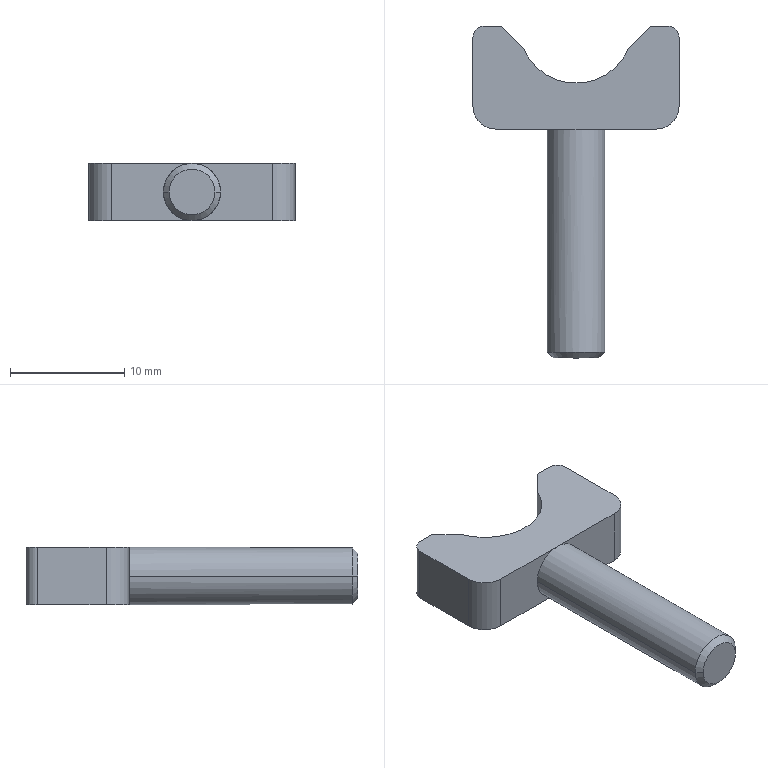Part | SolidWorks | features Chamfer 2, Fillet 2, ICE 2, Extrusion 1 | 1 solid | 20 faces | box 18 x 29 x 5 mm | volume 980.993 mm3 | plane 11 | cylinder 7 | cone 2 | commonest cylinder face diameters 2 x2 4 x2 5 x2 10 x1
STEP:
#1=CARTESIAN_POINT('',(2.,-29.,0.));
#2=VERTEX_POINT('',#1);
#3=CARTESIAN_POINT('',(-2.,-29.,0.));
#4=VERTEX_POINT('',#3);
#5=CARTESIAN_POINT('',(0.,-29.,0.));
#6=DIRECTION('',(0.,-1.,0.));
#7=DIRECTION('',(1.,0.,0.));
#8=AXIS2_PLACEMENT_3D('',#5,#6,#7);
#9=CIRCLE('',#8,2.);
#10=EDGE_CURVE('',#2,#4,#9,.T.);
#11=ORIENTED_EDGE('',*,*,#10,.F.);
#12=CARTESIAN_POINT('',(2.5,-28.5,0.));
#13=VERTEX_POINT('',#12);
#14=CARTESIAN_POINT('',(2.,-29.,0.));
#15=DIRECTION('',(0.7071,0.7071,0.));
#16=VECTOR('',#15,1000.);
#17=LINE('',#14,#16);
#18=EDGE_CURVE('',#2,#13,#17,.T.);
#19=ORIENTED_EDGE('',*,*,#18,.T.);
#20=CARTESIAN_POINT('',(-2.5,-28.5,0.));
#21=VERTEX_POINT('',#20);
#22=CARTESIAN_POINT('',(0.,-28.5,0.));
#23=DIRECTION('',(0.,1.,0.));
#24=DIRECTION('',(1.,0.,0.));
#25=AXIS2_PLACEMENT_3D('',#22,#23,#24);
#26=CIRCLE('',#25,2.5);
#27=EDGE_CURVE('',#21,#13,#26,.T.);
#28=ORIENTED_EDGE('',*,*,#27,.F.);
#29=CARTESIAN_POINT('',(-2.,-29.,0.));
#30=DIRECTION('',(-0.7071,0.7071,0.));
#31=VECTOR('',#30,1000.);
#32=LINE('',#29,#31);
#33=EDGE_CURVE('',#4,#21,#32,.T.);
#34=ORIENTED_EDGE('',*,*,#33,.F.);
#35=EDGE_LOOP('',(#11,#19,#28,#34));
#36=FACE_OUTER_BOUND('',#35,.T.);
#37=CARTESIAN_POINT('',(0.,-29.,0.));
#38=DIRECTION('',(0.,1.,0.));
#39=DIRECTION('',(-1.,0.,0.));
#40=AXIS2_PLACEMENT_3D('',#37,#38,#39);
#41=CONICAL_SURFACE('',#40,2.,0.7854);
#42=ADVANCED_FACE('',(#36),#41,.T.);
#43=ORIENTED_EDGE('',*,*,#27,.T.);
#44=CARTESIAN_POINT('',(2.5,-9.,0.));
#45=VERTEX_POINT('',#44);
#46=CARTESIAN_POINT('',(2.5,-29.,0.));
#47=DIRECTION('',(0.,1.,0.));
#48=VECTOR('',#47,1000.);
#49=LINE('',#46,#48);
#50=EDGE_CURVE('',#13,#45,#49,.T.);
#51=ORIENTED_EDGE('',*,*,#50,.T.);
#52=CARTESIAN_POINT('',(0.,-9.,2.5));
#53=VERTEX_POINT('',#52);
#54=CARTESIAN_POINT('',(0.,-9.,0.));
#55=DIRECTION('',(0.,-1.,0.));
#56=DIRECTION('',(1.,0.,0.));
#57=AXIS2_PLACEMENT_3D('',#54,#55,#56);
#58=CIRCLE('',#57,2.5);
#59=EDGE_CURVE('',#45,#53,#58,.T.);
#60=ORIENTED_EDGE('',*,*,#59,.T.);
#61=CARTESIAN_POINT('',(-2.5,-9.,0.));
#62=VERTEX_POINT('',#61);
#63=CARTESIAN_POINT('',(0.,-9.,0.));
#64=DIRECTION('',(0.,-1.,0.));
#65=DIRECTION('',(1.,0.,0.));
#66=AXIS2_PLACEMENT_3D('',#63,#64,#65);
#67=CIRCLE('',#66,2.5);
#68=EDGE_CURVE('',#53,#62,#67,.T.);
#69=ORIENTED_EDGE('',*,*,#68,.T.);
#70=CARTESIAN_POINT('',(-2.5,-29.,0.));
#71=DIRECTION('',(0.,1.,0.));
#72=VECTOR('',#71,1000.);
#73=LINE('',#70,#72);
#74=EDGE_CURVE('',#21,#62,#73,.T.);
#75=ORIENTED_EDGE('',*,*,#74,.F.);
#76=EDGE_LOOP('',(#43,#51,#60,#69,#75));
#77=FACE_OUTER_BOUND('',#76,.T.);
#78=CARTESIAN_POINT('',(0.,-29.,0.));
#79=DIRECTION('',(0.,1.,0.));
#80=DIRECTION('',(-1.,0.,0.));
#81=AXIS2_PLACEMENT_3D('',#78,#79,#80);
#82=CYLINDRICAL_SURFACE('',#81,2.5);
#83=ADVANCED_FACE('',(#77),#82,.T.);
#84=CARTESIAN_POINT('',(-7.,-9.,2.5));
#85=VERTEX_POINT('',#84);
#86=CARTESIAN_POINT('',(9.,-9.,2.5));
#87=DIRECTION('',(1.,0.,0.));
#88=VECTOR('',#87,1000.);
#89=LINE('',#86,#88);
#90=EDGE_CURVE('',#85,#53,#89,.T.);
#91=ORIENTED_EDGE('',*,*,#90,.F.);
#92=CARTESIAN_POINT('',(-7.,-9.,-2.5));
#93=VERTEX_POINT('',#92);
#94=CARTESIAN_POINT('',(-7.,-9.,2.5));
#95=DIRECTION('',(0.,0.,-1.));
#96=VECTOR('',#95,1000.);
#97=LINE('',#94,#96);
#98=EDGE_CURVE('',#85,#93,#97,.T.);
#99=ORIENTED_EDGE('',*,*,#98,.T.);
#100=CARTESIAN_POINT('',(0.,-9.,-2.5));
#101=VERTEX_POINT('',#100);
#102=CARTESIAN_POINT('',(9.,-9.,-2.5));
#103=DIRECTION('',(1.,0.,0.));
#104=VECTOR('',#103,1000.);
#105=LINE('',#102,#104);
#106=EDGE_CURVE('',#93,#101,#105,.T.);
#107=ORIENTED_EDGE('',*,*,#106,.T.);
#108=CARTESIAN_POINT('',(0.,-9.,0.));
#109=DIRECTION('',(0.,-1.,0.));
#110=DIRECTION('',(1.,0.,0.));
#111=AXIS2_PLACEMENT_3D('',#108,#109,#110);
#112=CIRCLE('',#111,2.5);
#113=EDGE_CURVE('',#62,#101,#112,.T.);
#114=ORIENTED_EDGE('',*,*,#113,.F.);
#115=ORIENTED_EDGE('',*,*,#68,.F.);
#116=EDGE_LOOP('',(#91,#99,#107,#114,#115));
#117=FACE_OUTER_BOUND('',#116,.T.);
#118=CARTESIAN_POINT('',(9.,-9.,2.5));
#119=DIRECTION('',(0.,1.,0.));
#120=DIRECTION('',(-1.,0.,0.));
#121=AXIS2_PLACEMENT_3D('',#118,#119,#120);
#122=PLANE('',#121);
#123=ADVANCED_FACE('',(#117),#122,.F.);
#124=CARTESIAN_POINT('',(9.,-7.,2.5));
#125=VERTEX_POINT('',#124);
#126=CARTESIAN_POINT('',(9.,-1.,2.5));
#127=VERTEX_POINT('',#126);
#128=CARTESIAN_POINT('',(9.,-9.,2.5));
#129=DIRECTION('',(0.,1.,0.));
#130=VECTOR('',#129,1000.);
#131=LINE('',#128,#130);
#132=EDGE_CURVE('',#125,#127,#131,.T.);
#133=ORIENTED_EDGE('',*,*,#132,.T.);
#134=CARTESIAN_POINT('',(8.,0.,2.5));
#135=VERTEX_POINT('',#134);
#136=CARTESIAN_POINT('',(8.,-1.,2.5));
#137=DIRECTION('',(0.,0.,1.));
#138=DIRECTION('',(1.,0.,0.));
#139=AXIS2_PLACEMENT_3D('',#136,#137,#138);
#140=CIRCLE('',#139,1.);
#141=EDGE_CURVE('',#127,#135,#140,.T.);
#142=ORIENTED_EDGE('',*,*,#141,.T.);
#143=CARTESIAN_POINT('',(6.5,0.,2.5));
#144=VERTEX_POINT('',#143);
#145=CARTESIAN_POINT('',(-9.,0.,2.5));
#146=DIRECTION('',(1.,0.,0.));
#147=VECTOR('',#146,1000.);
#148=LINE('',#145,#147);
#149=EDGE_CURVE('',#144,#135,#148,.T.);
#150=ORIENTED_EDGE('',*,*,#149,.F.);
#151=CARTESIAN_POINT('',(4.642,-1.858,2.5));
#152=VERTEX_POINT('',#151);
#153=CARTESIAN_POINT('',(3.25,-3.25,2.5));
#154=DIRECTION('',(-0.7071,-0.7071,0.));
#155=VECTOR('',#154,1000.);
#156=LINE('',#153,#155);
#157=EDGE_CURVE('',#144,#152,#156,.T.);
#158=ORIENTED_EDGE('',*,*,#157,.T.);
#159=CARTESIAN_POINT('',(-4.642,-1.858,2.5));
#160=VERTEX_POINT('',#159);
#161=CARTESIAN_POINT('',(0.,0.,2.5));
#162=DIRECTION('',(0.,0.,1.));
#163=DIRECTION('',(1.,0.,0.));
#164=AXIS2_PLACEMENT_3D('',#161,#162,#163);
#165=CIRCLE('',#164,5.);
#166=EDGE_CURVE('',#160,#152,#165,.T.);
#167=ORIENTED_EDGE('',*,*,#166,.F.);
#168=CARTESIAN_POINT('',(-6.5,0.,2.5));
#169=VERTEX_POINT('',#168);
#170=CARTESIAN_POINT('',(-3.25,-3.25,2.5));
#171=DIRECTION('',(-0.7071,0.7071,0.));
#172=VECTOR('',#171,1000.);
#173=LINE('',#170,#172);
#174=EDGE_CURVE('',#160,#169,#173,.T.);
#175=ORIENTED_EDGE('',*,*,#174,.T.);
#176=CARTESIAN_POINT('',(-8.,0.,2.5));
#177=VERTEX_POINT('',#176);
#178=CARTESIAN_POINT('',(-9.,0.,2.5));
#179=DIRECTION('',(1.,0.,0.));
#180=VECTOR('',#179,1000.);
#181=LINE('',#178,#180);
#182=EDGE_CURVE('',#177,#169,#181,.T.);
#183=ORIENTED_EDGE('',*,*,#182,.F.);
#184=CARTESIAN_POINT('',(-9.,-1.,2.5));
#185=VERTEX_POINT('',#184);
#186=CARTESIAN_POINT('',(-8.,-1.,2.5));
#187=DIRECTION('',(0.,0.,1.));
#188=DIRECTION('',(1.,0.,0.));
#189=AXIS2_PLACEMENT_3D('',#186,#187,#188);
#190=CIRCLE('',#189,1.);
#191=EDGE_CURVE('',#177,#185,#190,.T.);
#192=ORIENTED_EDGE('',*,*,#191,.T.);
#193=CARTESIAN_POINT('',(-9.,-7.,2.5));
#194=VERTEX_POINT('',#193);
#195=CARTESIAN_POINT('',(-9.,-9.,2.5));
#196=DIRECTION('',(0.,-1.,0.));
#197=VECTOR('',#196,1000.);
#198=LINE('',#195,#197);
#199=EDGE_CURVE('',#185,#194,#198,.T.);
#200=ORIENTED_EDGE('',*,*,#199,.T.);
#201=CARTESIAN_POINT('',(-7.,-7.,2.5));
#202=DIRECTION('',(0.,0.,1.));
#203=DIRECTION('',(1.,0.,0.));
#204=AXIS2_PLACEMENT_3D('',#201,#202,#203);
#205=CIRCLE('',#204,2.);
#206=EDGE_CURVE('',#194,#85,#205,.T.);
#207=ORIENTED_EDGE('',*,*,#206,.T.);
#208=ORIENTED_EDGE('',*,*,#90,.T.);
#209=CARTESIAN_POINT('',(7.,-9.,2.5));
#210=VERTEX_POINT('',#209);
#211=CARTESIAN_POINT('',(9.,-9.,2.5));
#212=DIRECTION('',(1.,0.,0.));
#213=VECTOR('',#212,1000.);
#214=LINE('',#211,#213);
#215=EDGE_CURVE('',#53,#210,#214,.T.);
#216=ORIENTED_EDGE('',*,*,#215,.T.);
#217=CARTESIAN_POINT('',(7.,-7.,2.5));
#218=DIRECTION('',(0.,0.,1.));
#219=DIRECTION('',(1.,0.,0.));
#220=AXIS2_PLACEMENT_3D('',#217,#218,#219);
#221=CIRCLE('',#220,2.);
#222=EDGE_CURVE('',#210,#125,#221,.T.);
#223=ORIENTED_EDGE('',*,*,#222,.T.);
#224=EDGE_LOOP('',(#133,#142,#150,#158,#167,#175,#183,#192,#200,#207,#208,#216,#223));
#225=FACE_OUTER_BOUND('',#224,.T.);
#226=CARTESIAN_POINT('',(0.,0.,2.5));
#227=DIRECTION('',(0.,0.,1.));
#228=DIRECTION('',(1.,0.,0.));
#229=AXIS2_PLACEMENT_3D('',#226,#227,#228);
#230=PLANE('',#229);
#231=ADVANCED_FACE('',(#225),#230,.T.);
#232=CARTESIAN_POINT('',(6.5,0.,-2.5));
#233=VERTEX_POINT('',#232);
#234=CARTESIAN_POINT('',(8.,0.,-2.5));
#235=VERTEX_POINT('',#234);
#236=CARTESIAN_POINT('',(-9.,0.,-2.5));
#237=DIRECTION('',(1.,0.,0.));
#238=VECTOR('',#237,1000.);
#239=LINE('',#236,#238);
#240=EDGE_CURVE('',#233,#235,#239,.T.);
#241=ORIENTED_EDGE('',*,*,#240,.T.);
#242=CARTESIAN_POINT('',(9.,-1.,-2.5));
#243=VERTEX_POINT('',#242);
#244=CARTESIAN_POINT('',(8.,-1.,-2.5));
#245=DIRECTION('',(0.,0.,-1.));
#246=DIRECTION('',(1.,0.,0.));
#247=AXIS2_PLACEMENT_3D('',#244,#245,#246);
#248=CIRCLE('',#247,1.);
#249=EDGE_CURVE('',#235,#243,#248,.T.);
#250=ORIENTED_EDGE('',*,*,#249,.T.);
#251=CARTESIAN_POINT('',(9.,-7.,-2.5));
#252=VERTEX_POINT('',#251);
#253=CARTESIAN_POINT('',(9.,-9.,-2.5));
#254=DIRECTION('',(0.,1.,0.));
#255=VECTOR('',#254,1000.);
#256=LINE('',#253,#255);
#257=EDGE_CURVE('',#252,#243,#256,.T.);
#258=ORIENTED_EDGE('',*,*,#257,.F.);
#259=CARTESIAN_POINT('',(7.,-9.,-2.5));
#260=VERTEX_POINT('',#259);
#261=CARTESIAN_POINT('',(7.,-7.,-2.5));
#262=DIRECTION('',(0.,0.,-1.));
#263=DIRECTION('',(1.,0.,0.));
#264=AXIS2_PLACEMENT_3D('',#261,#262,#263);
#265=CIRCLE('',#264,2.);
#266=EDGE_CURVE('',#252,#260,#265,.T.);
#267=ORIENTED_EDGE('',*,*,#266,.T.);
#268=CARTESIAN_POINT('',(9.,-9.,-2.5));
#269=DIRECTION('',(1.,0.,0.));
#270=VECTOR('',#269,1000.);
#271=LINE('',#268,#270);
#272=EDGE_CURVE('',#101,#260,#271,.T.);
#273=ORIENTED_EDGE('',*,*,#272,.F.);
#274=ORIENTED_EDGE('',*,*,#106,.F.);
#275=CARTESIAN_POINT('',(-9.,-7.,-2.5));
#276=VERTEX_POINT('',#275);
#277=CARTESIAN_POINT('',(-7.,-7.,-2.5));
#278=DIRECTION('',(0.,0.,-1.));
#279=DIRECTION('',(1.,0.,0.));
#280=AXIS2_PLACEMENT_3D('',#277,#278,#279);
#281=CIRCLE('',#280,2.);
#282=EDGE_CURVE('',#93,#276,#281,.T.);
#283=ORIENTED_EDGE('',*,*,#282,.T.);
#284=CARTESIAN_POINT('',(-9.,-1.,-2.5));
#285=VERTEX_POINT('',#284);
#286=CARTESIAN_POINT('',(-9.,-9.,-2.5));
#287=DIRECTION('',(0.,-1.,0.));
#288=VECTOR('',#287,1000.);
#289=LINE('',#286,#288);
#290=EDGE_CURVE('',#285,#276,#289,.T.);
#291=ORIENTED_EDGE('',*,*,#290,.F.);
#292=CARTESIAN_POINT('',(-8.,0.,-2.5));
#293=VERTEX_POINT('',#292);
#294=CARTESIAN_POINT('',(-8.,-1.,-2.5));
#295=DIRECTION('',(0.,0.,-1.));
#296=DIRECTION('',(1.,0.,0.));
#297=AXIS2_PLACEMENT_3D('',#294,#295,#296);
#298=CIRCLE('',#297,1.);
#299=EDGE_CURVE('',#285,#293,#298,.T.);
#300=ORIENTED_EDGE('',*,*,#299,.T.);
#301=CARTESIAN_POINT('',(-6.5,0.,-2.5));
#302=VERTEX_POINT('',#301);
#303=CARTESIAN_POINT('',(-9.,0.,-2.5));
#304=DIRECTION('',(1.,0.,0.));
#305=VECTOR('',#304,1000.);
#306=LINE('',#303,#305);
#307=EDGE_CURVE('',#293,#302,#306,.T.);
#308=ORIENTED_EDGE('',*,*,#307,.T.);
#309=CARTESIAN_POINT('',(-4.642,-1.858,-2.5));
#310=VERTEX_POINT('',#309);
#311=CARTESIAN_POINT('',(-6.5,0.,-2.5));
#312=DIRECTION('',(0.7071,-0.7071,0.));
#313=VECTOR('',#312,1000.);
#314=LINE('',#311,#313);
#315=EDGE_CURVE('',#302,#310,#314,.T.);
#316=ORIENTED_EDGE('',*,*,#315,.T.);
#317=CARTESIAN_POINT('',(4.642,-1.858,-2.5));
#318=VERTEX_POINT('',#317);
#319=CARTESIAN_POINT('',(0.,0.,-2.5));
#320=DIRECTION('',(0.,0.,1.));
#321=DIRECTION('',(1.,0.,0.));
#322=AXIS2_PLACEMENT_3D('',#319,#320,#321);
#323=CIRCLE('',#322,5.);
#324=EDGE_CURVE('',#310,#318,#323,.T.);
#325=ORIENTED_EDGE('',*,*,#324,.T.);
#326=CARTESIAN_POINT('',(6.5,0.,-2.5));
#327=DIRECTION('',(0.7071,0.7071,0.));
#328=VECTOR('',#327,1000.);
#329=LINE('',#326,#328);
#330=EDGE_CURVE('',#318,#233,#329,.T.);
#331=ORIENTED_EDGE('',*,*,#330,.T.);
#332=EDGE_LOOP('',(#241,#250,#258,#267,#273,#274,#283,#291,#300,#308,#316,#325,#331));
#333=FACE_OUTER_BOUND('',#332,.T.);
#334=CARTESIAN_POINT('',(0.,0.,-2.5));
#335=DIRECTION('',(0.,0.,1.));
#336=DIRECTION('',(1.,0.,0.));
#337=AXIS2_PLACEMENT_3D('',#334,#335,#336);
#338=PLANE('',#337);
#339=ADVANCED_FACE('',(#333),#338,.F.);
#340=ORIENTED_EDGE('',*,*,#199,.F.);
#341=CARTESIAN_POINT('',(-9.,-1.,2.5));
#342=DIRECTION('',(0.,0.,-1.));
#343=VECTOR('',#342,1000.);
#344=LINE('',#341,#343);
#345=EDGE_CURVE('',#185,#285,#344,.T.);
#346=ORIENTED_EDGE('',*,*,#345,.T.);
#347=ORIENTED_EDGE('',*,*,#290,.T.);
#348=CARTESIAN_POINT('',(-9.,-7.,2.5));
#349=DIRECTION('',(0.,0.,1.));
#350=VECTOR('',#349,1000.);
#351=LINE('',#348,#350);
#352=EDGE_CURVE('',#276,#194,#351,.T.);
#353=ORIENTED_EDGE('',*,*,#352,.T.);
#354=EDGE_LOOP('',(#340,#346,#347,#353));
#355=FACE_OUTER_BOUND('',#354,.T.);
#356=CARTESIAN_POINT('',(-9.,-9.,2.5));
#357=DIRECTION('',(1.,0.,0.));
#358=DIRECTION('',(0.,0.,-1.));
#359=AXIS2_PLACEMENT_3D('',#356,#357,#358);
#360=PLANE('',#359);
#361=ADVANCED_FACE('',(#355),#360,.F.);
#362=ORIENTED_EDGE('',*,*,#272,.T.);
#363=CARTESIAN_POINT('',(7.,-9.,2.5));
#364=DIRECTION('',(0.,0.,1.));
#365=VECTOR('',#364,1000.);
#366=LINE('',#363,#365);
#367=EDGE_CURVE('',#260,#210,#366,.T.);
#368=ORIENTED_EDGE('',*,*,#367,.T.);
#369=ORIENTED_EDGE('',*,*,#215,.F.);
#370=ORIENTED_EDGE('',*,*,#59,.F.);
#371=CARTESIAN_POINT('',(0.,-9.,0.));
#372=DIRECTION('',(0.,-1.,0.));
#373=DIRECTION('',(1.,0.,0.));
#374=AXIS2_PLACEMENT_3D('',#371,#372,#373);
#375=CIRCLE('',#374,2.5);
#376=EDGE_CURVE('',#101,#45,#375,.T.);
#377=ORIENTED_EDGE('',*,*,#376,.F.);
#378=EDGE_LOOP('',(#362,#368,#369,#370,#377));
#379=FACE_OUTER_BOUND('',#378,.T.);
#380=CARTESIAN_POINT('',(9.,-9.,2.5));
#381=DIRECTION('',(0.,1.,0.));
#382=DIRECTION('',(-1.,0.,0.));
#383=AXIS2_PLACEMENT_3D('',#380,#381,#382);
#384=PLANE('',#383);
#385=ADVANCED_FACE('',(#379),#384,.F.);
#386=ORIENTED_EDGE('',*,*,#257,.T.);
#387=CARTESIAN_POINT('',(9.,-1.,2.5));
#388=DIRECTION('',(0.,0.,1.));
#389=VECTOR('',#388,1000.);
#390=LINE('',#387,#389);
#391=EDGE_CURVE('',#243,#127,#390,.T.);
#392=ORIENTED_EDGE('',*,*,#391,.T.);
#393=ORIENTED_EDGE('',*,*,#132,.F.);
#394=CARTESIAN_POINT('',(9.,-7.,2.5));
#395=DIRECTION('',(0.,0.,-1.));
#396=VECTOR('',#395,1000.);
#397=LINE('',#394,#396);
#398=EDGE_CURVE('',#125,#252,#397,.T.);
#399=ORIENTED_EDGE('',*,*,#398,.T.);
#400=EDGE_LOOP('',(#386,#392,#393,#399));
#401=FACE_OUTER_BOUND('',#400,.T.);
#402=CARTESIAN_POINT('',(9.,-9.,2.5));
#403=DIRECTION('',(-1.,0.,0.));
#404=DIRECTION('',(0.,-1.,0.));
#405=AXIS2_PLACEMENT_3D('',#402,#403,#404);
#406=PLANE('',#405);
#407=ADVANCED_FACE('',(#401),#406,.F.);
#408=ORIENTED_EDGE('',*,*,#166,.T.);
#409=CARTESIAN_POINT('',(4.642,-1.858,2.5));
#410=DIRECTION('',(0.,0.,-1.));
#411=VECTOR('',#410,1000.);
#412=LINE('',#409,#411);
#413=EDGE_CURVE('',#152,#318,#412,.T.);
#414=ORIENTED_EDGE('',*,*,#413,.T.);
#415=ORIENTED_EDGE('',*,*,#324,.F.);
#416=CARTESIAN_POINT('',(-4.642,-1.858,2.5));
#417=DIRECTION('',(0.,0.,1.));
#418=VECTOR('',#417,1000.);
#419=LINE('',#416,#418);
#420=EDGE_CURVE('',#310,#160,#419,.T.);
#421=ORIENTED_EDGE('',*,*,#420,.T.);
#422=EDGE_LOOP('',(#408,#414,#415,#421));
#423=FACE_OUTER_BOUND('',#422,.T.);
#424=CARTESIAN_POINT('',(0.,0.,2.5));
#425=DIRECTION('',(0.,0.,-1.));
#426=DIRECTION('',(-1.,0.,0.));
#427=AXIS2_PLACEMENT_3D('',#424,#425,#426);
#428=CYLINDRICAL_SURFACE('',#427,5.);
#429=ADVANCED_FACE('',(#423),#428,.F.);
#430=ORIENTED_EDGE('',*,*,#50,.F.);
#431=CARTESIAN_POINT('',(0.,-28.5,0.));
#432=DIRECTION('',(0.,1.,0.));
#433=DIRECTION('',(1.,0.,0.));
#434=AXIS2_PLACEMENT_3D('',#431,#432,#433);
#435=CIRCLE('',#434,2.5);
#436=EDGE_CURVE('',#13,#21,#435,.T.);
#437=ORIENTED_EDGE('',*,*,#436,.T.);
#438=ORIENTED_EDGE('',*,*,#74,.T.);
#439=ORIENTED_EDGE('',*,*,#113,.T.);
#440=ORIENTED_EDGE('',*,*,#376,.T.);
#441=EDGE_LOOP('',(#430,#437,#438,#439,#440));
#442=FACE_OUTER_BOUND('',#441,.T.);
#443=CARTESIAN_POINT('',(0.,-29.,0.));
#444=DIRECTION('',(0.,1.,0.));
#445=DIRECTION('',(-1.,0.,0.));
#446=AXIS2_PLACEMENT_3D('',#443,#444,#445);
#447=CYLINDRICAL_SURFACE('',#446,2.5);
#448=ADVANCED_FACE('',(#442),#447,.T.);
#449=CARTESIAN_POINT('',(0.,-29.,0.));
#450=DIRECTION('',(0.,-1.,0.));
#451=DIRECTION('',(1.,0.,0.));
#452=AXIS2_PLACEMENT_3D('',#449,#450,#451);
#453=CIRCLE('',#452,2.);
#454=EDGE_CURVE('',#4,#2,#453,.T.);
#455=ORIENTED_EDGE('',*,*,#454,.T.);
#456=ORIENTED_EDGE('',*,*,#10,.T.);
#457=EDGE_LOOP('',(#455,#456));
#458=FACE_OUTER_BOUND('',#457,.T.);
#459=CARTESIAN_POINT('',(0.,-29.,0.));
#460=DIRECTION('',(0.,-1.,0.));
#461=DIRECTION('',(1.,0.,0.));
#462=AXIS2_PLACEMENT_3D('',#459,#460,#461);
#463=PLANE('',#462);
#464=ADVANCED_FACE('',(#458),#463,.T.);
#465=ORIENTED_EDGE('',*,*,#149,.T.);
#466=CARTESIAN_POINT('',(8.,0.,-2.5));
#467=DIRECTION('',(0.,0.,-1.));
#468=VECTOR('',#467,1000.);
#469=LINE('',#466,#468);
#470=EDGE_CURVE('',#135,#235,#469,.T.);
#471=ORIENTED_EDGE('',*,*,#470,.T.);
#472=ORIENTED_EDGE('',*,*,#240,.F.);
#473=CARTESIAN_POINT('',(6.5,0.,2.5));
#474=DIRECTION('',(0.,0.,1.));
#475=VECTOR('',#474,1000.);
#476=LINE('',#473,#475);
#477=EDGE_CURVE('',#233,#144,#476,.T.);
#478=ORIENTED_EDGE('',*,*,#477,.T.);
#479=EDGE_LOOP('',(#465,#471,#472,#478));
#480=FACE_OUTER_BOUND('',#479,.T.);
#481=CARTESIAN_POINT('',(-9.,0.,-2.5));
#482=DIRECTION('',(0.,-1.,0.));
#483=DIRECTION('',(0.,0.,-1.));
#484=AXIS2_PLACEMENT_3D('',#481,#482,#483);
#485=PLANE('',#484);
#486=ADVANCED_FACE('',(#480),#485,.F.);
#487=ORIENTED_EDGE('',*,*,#307,.F.);
#488=CARTESIAN_POINT('',(-8.,0.,-2.5));
#489=DIRECTION('',(0.,0.,1.));
#490=VECTOR('',#489,1000.);
#491=LINE('',#488,#490);
#492=EDGE_CURVE('',#293,#177,#491,.T.);
#493=ORIENTED_EDGE('',*,*,#492,.T.);
#494=ORIENTED_EDGE('',*,*,#182,.T.);
#495=CARTESIAN_POINT('',(-6.5,0.,-2.5));
#496=DIRECTION('',(0.,0.,-1.));
#497=VECTOR('',#496,1000.);
#498=LINE('',#495,#497);
#499=EDGE_CURVE('',#169,#302,#498,.T.);
#500=ORIENTED_EDGE('',*,*,#499,.T.);
#501=EDGE_LOOP('',(#487,#493,#494,#500));
#502=FACE_OUTER_BOUND('',#501,.T.);
#503=CARTESIAN_POINT('',(-9.,0.,-2.5));
#504=DIRECTION('',(0.,-1.,0.));
#505=DIRECTION('',(0.,0.,-1.));
#506=AXIS2_PLACEMENT_3D('',#503,#504,#505);
#507=PLANE('',#506);
#508=ADVANCED_FACE('',(#502),#507,.F.);
#509=ORIENTED_EDGE('',*,*,#330,.F.);
#510=ORIENTED_EDGE('',*,*,#413,.F.);
#511=ORIENTED_EDGE('',*,*,#157,.F.);
#512=ORIENTED_EDGE('',*,*,#477,.F.);
#513=EDGE_LOOP('',(#509,#510,#511,#512));
#514=FACE_OUTER_BOUND('',#513,.T.);
#515=CARTESIAN_POINT('',(6.5,0.,2.5));
#516=DIRECTION('',(-0.7071,0.7071,0.));
#517=DIRECTION('',(0.,0.,-1.));
#518=AXIS2_PLACEMENT_3D('',#515,#516,#517);
#519=PLANE('',#518);
#520=ADVANCED_FACE('',(#514),#519,.T.);
#521=ORIENTED_EDGE('',*,*,#174,.F.);
#522=ORIENTED_EDGE('',*,*,#420,.F.);
#523=ORIENTED_EDGE('',*,*,#315,.F.);
#524=ORIENTED_EDGE('',*,*,#499,.F.);
#525=EDGE_LOOP('',(#521,#522,#523,#524));
#526=FACE_OUTER_BOUND('',#525,.T.);
#527=CARTESIAN_POINT('',(-6.5,0.,2.5));
#528=DIRECTION('',(-0.7071,-0.7071,0.));
#529=DIRECTION('',(0.,0.,-1.));
#530=AXIS2_PLACEMENT_3D('',#527,#528,#529);
#531=PLANE('',#530);
#532=ADVANCED_FACE('',(#526),#531,.F.);
#533=ORIENTED_EDGE('',*,*,#222,.F.);
#534=ORIENTED_EDGE('',*,*,#367,.F.);
#535=ORIENTED_EDGE('',*,*,#266,.F.);
#536=ORIENTED_EDGE('',*,*,#398,.F.);
#537=EDGE_LOOP('',(#533,#534,#535,#536));
#538=FACE_OUTER_BOUND('',#537,.T.);
#539=CARTESIAN_POINT('',(7.,-7.,2.5));
#540=DIRECTION('',(0.,0.,-1.));
#541=DIRECTION('',(-1.,0.,0.));
#542=AXIS2_PLACEMENT_3D('',#539,#540,#541);
#543=CYLINDRICAL_SURFACE('',#542,2.);
#544=ADVANCED_FACE('',(#538),#543,.T.);
#545=ORIENTED_EDGE('',*,*,#206,.F.);
#546=ORIENTED_EDGE('',*,*,#352,.F.);
#547=ORIENTED_EDGE('',*,*,#282,.F.);
#548=ORIENTED_EDGE('',*,*,#98,.F.);
#549=EDGE_LOOP('',(#545,#546,#547,#548));
#550=FACE_OUTER_BOUND('',#549,.T.);
#551=CARTESIAN_POINT('',(-7.,-7.,2.5));
#552=DIRECTION('',(0.,0.,-1.));
#553=DIRECTION('',(-1.,0.,0.));
#554=AXIS2_PLACEMENT_3D('',#551,#552,#553);
#555=CYLINDRICAL_SURFACE('',#554,2.);
#556=ADVANCED_FACE('',(#550),#555,.T.);
#557=ORIENTED_EDGE('',*,*,#249,.F.);
#558=ORIENTED_EDGE('',*,*,#470,.F.);
#559=ORIENTED_EDGE('',*,*,#141,.F.);
#560=ORIENTED_EDGE('',*,*,#391,.F.);
#561=EDGE_LOOP('',(#557,#558,#559,#560));
#562=FACE_OUTER_BOUND('',#561,.T.);
#563=CARTESIAN_POINT('',(8.,-1.,2.5));
#564=DIRECTION('',(0.,0.,1.));
#565=DIRECTION('',(1.,0.,0.));
#566=AXIS2_PLACEMENT_3D('',#563,#564,#565);
#567=CYLINDRICAL_SURFACE('',#566,1.);
#568=ADVANCED_FACE('',(#562),#567,.T.);
#569=ORIENTED_EDGE('',*,*,#299,.F.);
#570=ORIENTED_EDGE('',*,*,#345,.F.);
#571=ORIENTED_EDGE('',*,*,#191,.F.);
#572=ORIENTED_EDGE('',*,*,#492,.F.);
#573=EDGE_LOOP('',(#569,#570,#571,#572));
#574=FACE_OUTER_BOUND('',#573,.T.);
#575=CARTESIAN_POINT('',(-8.,-1.,-2.5));
#576=DIRECTION('',(0.,0.,1.));
#577=DIRECTION('',(1.,0.,0.));
#578=AXIS2_PLACEMENT_3D('',#575,#576,#577);
#579=CYLINDRICAL_SURFACE('',#578,1.);
#580=ADVANCED_FACE('',(#574),#579,.T.);
#581=ORIENTED_EDGE('',*,*,#18,.F.);
#582=ORIENTED_EDGE('',*,*,#454,.F.);
#583=ORIENTED_EDGE('',*,*,#33,.T.);
#584=ORIENTED_EDGE('',*,*,#436,.F.);
#585=EDGE_LOOP('',(#581,#582,#583,#584));
#586=FACE_OUTER_BOUND('',#585,.T.);
#587=CARTESIAN_POINT('',(0.,-29.,0.));
#588=DIRECTION('',(0.,1.,0.));
#589=DIRECTION('',(-1.,0.,0.));
#590=AXIS2_PLACEMENT_3D('',#587,#588,#589);
#591=CONICAL_SURFACE('',#590,2.,0.7854);
#592=ADVANCED_FACE('',(#586),#591,.T.);
#593=CLOSED_SHELL('',(#42,#83,#123,#231,#339,#361,#385,#407,#429,#448,#464,#486,#508,#520,#532,#544,#556,#568,#580,#592));
#594=MANIFOLD_SOLID_BREP('',#593);
#595=CARTESIAN_POINT('',(0.,0.,0.));
#596=DIRECTION('',(0.,0.,1.));
#597=DIRECTION('',(1.,0.,0.));
#598=AXIS2_PLACEMENT_3D('',#595,#596,#597);
#599=(LENGTH_UNIT()NAMED_UNIT(*)SI_UNIT(.MILLI.,.METRE.));
#600=UNCERTAINTY_MEASURE_WITH_UNIT(LENGTH_MEASURE(0.00001),#599,'','');
#601=(NAMED_UNIT(*)PLANE_ANGLE_UNIT()SI_UNIT($,.RADIAN.));
#602=(NAMED_UNIT(*)SI_UNIT($,.STERADIAN.)SOLID_ANGLE_UNIT());
#603=(GEOMETRIC_REPRESENTATION_CONTEXT(3)GLOBAL_UNCERTAINTY_ASSIGNED_CONTEXT((#600))GLOBAL_UNIT_ASSIGNED_CONTEXT((#599,#601,#602))REPRESENTATION_CONTEXT('',''));
#604=ADVANCED_BREP_SHAPE_REPRESENTATION('',(#594,#598),#603);